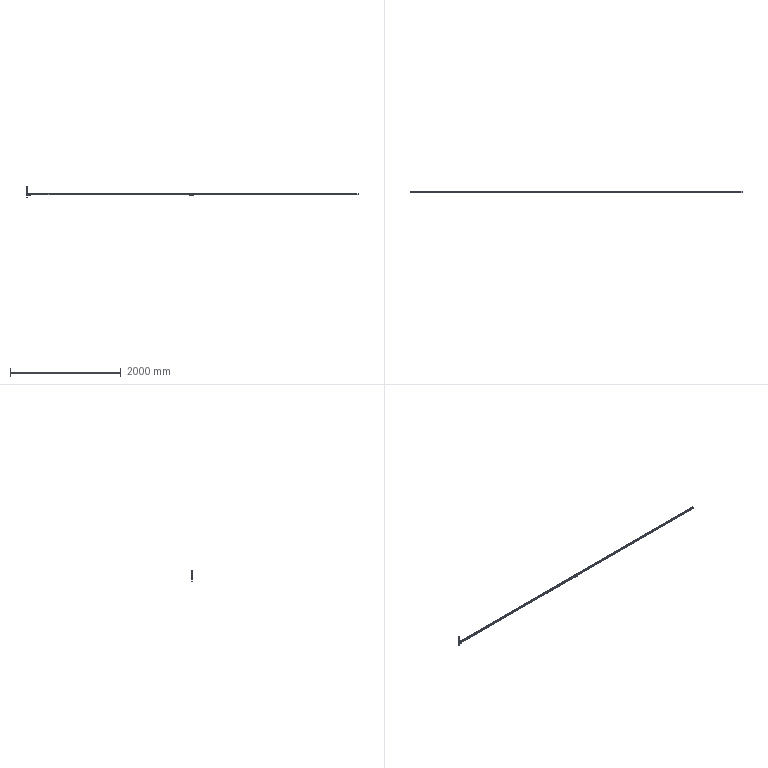Part | STEP file | ASND-0110-Q1 | 1 solid | 479 faces | box 5993 x 32 x 186 mm | volume 1783036 mm3 | plane 301 | cylinder 144 | cone 32 | other 2 | commonest cylinder face diameters 32 x22 24 x18 31 x18 4.134 x16 12 x14 6 x8